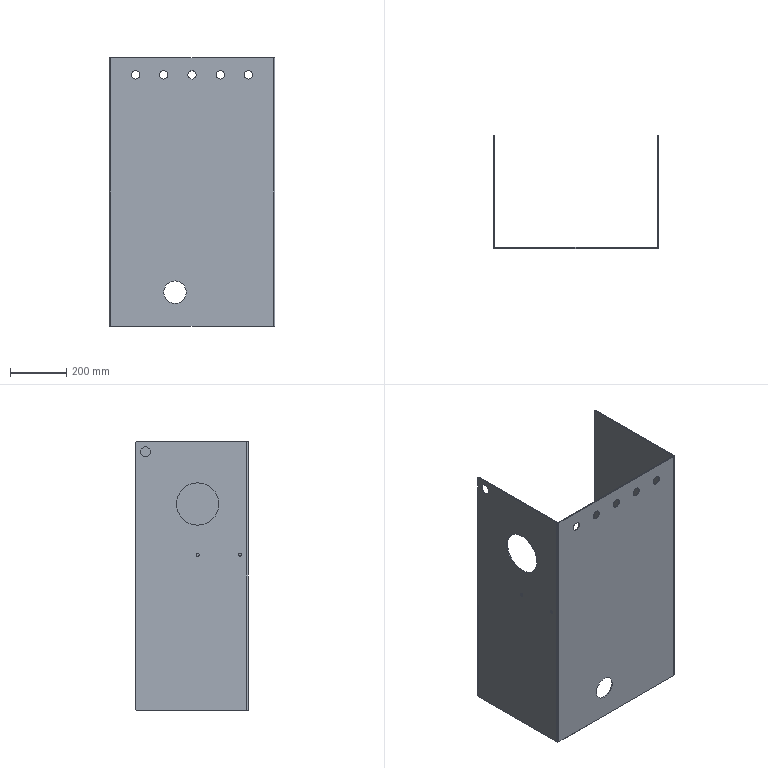Part | SolidWorks | features ICE 4, FlatPattern 1, SMBaseFlange 1, SheetMetal 1 | 1 solid | 48 faces | box 586 x 400 x 950 mm | volume 3763524 mm3 | cylinder 30 | plane 18 | commonest cylinder face diameters 30 x10 6 x6 10.5 x4 12 x2 35 x2 80 x2
STEP:
#1=CARTESIAN_POINT('',(583.,290.,140.));
#2=VERTEX_POINT('',#1);
#3=CARTESIAN_POINT('',(583.,290.,320.));
#4=VERTEX_POINT('',#3);
#5=CARTESIAN_POINT('',(583.,290.,230.));
#6=DIRECTION('',(-1.,0.,0.));
#7=DIRECTION('',(0.,0.,1.));
#8=AXIS2_PLACEMENT_3D('',#5,#6,#7);
#9=CIRCLE('',#8,90.);
#10=EDGE_CURVE('',#2,#4,#9,.T.);
#11=ORIENTED_EDGE('',*,*,#10,.T.);
#12=CARTESIAN_POINT('',(586.,290.,320.));
#13=VERTEX_POINT('',#12);
#14=CARTESIAN_POINT('',(576.,290.,320.));
#15=DIRECTION('',(1.,0.,0.));
#16=VECTOR('',#15,1000.);
#17=LINE('',#14,#16);
#18=EDGE_CURVE('',#4,#13,#17,.T.);
#19=ORIENTED_EDGE('',*,*,#18,.T.);
#20=CARTESIAN_POINT('',(586.,290.,140.));
#21=VERTEX_POINT('',#20);
#22=CARTESIAN_POINT('',(586.,290.,230.));
#23=DIRECTION('',(1.,0.,0.));
#24=DIRECTION('',(0.,0.,-1.));
#25=AXIS2_PLACEMENT_3D('',#22,#23,#24);
#26=CIRCLE('',#25,90.);
#27=EDGE_CURVE('',#13,#21,#26,.T.);
#28=ORIENTED_EDGE('',*,*,#27,.T.);
#29=CARTESIAN_POINT('',(576.,290.,140.));
#30=DIRECTION('',(1.,0.,0.));
#31=VECTOR('',#30,1000.);
#32=LINE('',#29,#31);
#33=EDGE_CURVE('',#2,#21,#32,.T.);
#34=ORIENTED_EDGE('',*,*,#33,.F.);
#35=EDGE_LOOP('',(#11,#19,#28,#34));
#36=FACE_OUTER_BOUND('',#35,.T.);
#37=CARTESIAN_POINT('',(576.,290.,230.));
#38=DIRECTION('',(1.,0.,0.));
#39=DIRECTION('',(0.,0.,-1.));
#40=AXIS2_PLACEMENT_3D('',#37,#38,#39);
#41=CYLINDRICAL_SURFACE('',#40,90.);
#42=ADVANCED_FACE('',(#36),#41,.F.);
#43=CARTESIAN_POINT('',(233.,3.,80.));
#44=VERTEX_POINT('',#43);
#45=CARTESIAN_POINT('',(233.,3.,160.));
#46=VERTEX_POINT('',#45);
#47=CARTESIAN_POINT('',(233.,3.,120.));
#48=DIRECTION('',(0.,1.,0.));
#49=DIRECTION('',(0.,0.,1.));
#50=AXIS2_PLACEMENT_3D('',#47,#48,#49);
#51=CIRCLE('',#50,40.);
#52=EDGE_CURVE('',#44,#46,#51,.T.);
#53=ORIENTED_EDGE('',*,*,#52,.T.);
#54=CARTESIAN_POINT('',(233.,0.,160.));
#55=VERTEX_POINT('',#54);
#56=CARTESIAN_POINT('',(233.,10.,160.));
#57=DIRECTION('',(0.,-1.,0.));
#58=VECTOR('',#57,1000.);
#59=LINE('',#56,#58);
#60=EDGE_CURVE('',#46,#55,#59,.T.);
#61=ORIENTED_EDGE('',*,*,#60,.T.);
#62=CARTESIAN_POINT('',(233.,0.,80.));
#63=VERTEX_POINT('',#62);
#64=CARTESIAN_POINT('',(233.,0.,120.));
#65=DIRECTION('',(0.,-1.,0.));
#66=DIRECTION('',(0.,0.,-1.));
#67=AXIS2_PLACEMENT_3D('',#64,#65,#66);
#68=CIRCLE('',#67,40.);
#69=EDGE_CURVE('',#55,#63,#68,.T.);
#70=ORIENTED_EDGE('',*,*,#69,.T.);
#71=CARTESIAN_POINT('',(233.,10.,80.));
#72=DIRECTION('',(0.,-1.,0.));
#73=VECTOR('',#72,1000.);
#74=LINE('',#71,#73);
#75=EDGE_CURVE('',#44,#63,#74,.T.);
#76=ORIENTED_EDGE('',*,*,#75,.F.);
#77=EDGE_LOOP('',(#53,#61,#70,#76));
#78=FACE_OUTER_BOUND('',#77,.T.);
#79=CARTESIAN_POINT('',(233.,10.,120.));
#80=DIRECTION('',(0.,-1.,0.));
#81=DIRECTION('',(0.,0.,-1.));
#82=AXIS2_PLACEMENT_3D('',#79,#80,#81);
#83=CYLINDRICAL_SURFACE('',#82,40.);
#84=ADVANCED_FACE('',(#78),#83,.F.);
#85=CARTESIAN_POINT('',(493.,3.,875.));
#86=VERTEX_POINT('',#85);
#87=CARTESIAN_POINT('',(493.,3.,905.));
#88=VERTEX_POINT('',#87);
#89=CARTESIAN_POINT('',(493.,3.,890.));
#90=DIRECTION('',(0.,1.,0.));
#91=DIRECTION('',(0.,0.,1.));
#92=AXIS2_PLACEMENT_3D('',#89,#90,#91);
#93=CIRCLE('',#92,15.);
#94=EDGE_CURVE('',#86,#88,#93,.T.);
#95=ORIENTED_EDGE('',*,*,#94,.T.);
#96=CARTESIAN_POINT('',(493.,0.,905.));
#97=VERTEX_POINT('',#96);
#98=CARTESIAN_POINT('',(493.,10.,905.));
#99=DIRECTION('',(0.,-1.,0.));
#100=VECTOR('',#99,1000.);
#101=LINE('',#98,#100);
#102=EDGE_CURVE('',#88,#97,#101,.T.);
#103=ORIENTED_EDGE('',*,*,#102,.T.);
#104=CARTESIAN_POINT('',(493.,0.,875.));
#105=VERTEX_POINT('',#104);
#106=CARTESIAN_POINT('',(493.,0.,890.));
#107=DIRECTION('',(0.,-1.,0.));
#108=DIRECTION('',(0.,0.,-1.));
#109=AXIS2_PLACEMENT_3D('',#106,#107,#108);
#110=CIRCLE('',#109,15.);
#111=EDGE_CURVE('',#97,#105,#110,.T.);
#112=ORIENTED_EDGE('',*,*,#111,.T.);
#113=CARTESIAN_POINT('',(493.,10.,875.));
#114=DIRECTION('',(0.,-1.,0.));
#115=VECTOR('',#114,1000.);
#116=LINE('',#113,#115);
#117=EDGE_CURVE('',#86,#105,#116,.T.);
#118=ORIENTED_EDGE('',*,*,#117,.F.);
#119=EDGE_LOOP('',(#95,#103,#112,#118));
#120=FACE_OUTER_BOUND('',#119,.T.);
#121=CARTESIAN_POINT('',(493.,10.,890.));
#122=DIRECTION('',(0.,-1.,0.));
#123=DIRECTION('',(0.,0.,-1.));
#124=AXIS2_PLACEMENT_3D('',#121,#122,#123);
#125=CYLINDRICAL_SURFACE('',#124,15.);
#126=ADVANCED_FACE('',(#120),#125,.F.);
#127=CARTESIAN_POINT('',(393.,3.,875.));
#128=VERTEX_POINT('',#127);
#129=CARTESIAN_POINT('',(393.,3.,905.));
#130=VERTEX_POINT('',#129);
#131=CARTESIAN_POINT('',(393.,3.,890.));
#132=DIRECTION('',(0.,1.,0.));
#133=DIRECTION('',(0.,0.,1.));
#134=AXIS2_PLACEMENT_3D('',#131,#132,#133);
#135=CIRCLE('',#134,15.);
#136=EDGE_CURVE('',#128,#130,#135,.T.);
#137=ORIENTED_EDGE('',*,*,#136,.T.);
#138=CARTESIAN_POINT('',(393.,0.,905.));
#139=VERTEX_POINT('',#138);
#140=CARTESIAN_POINT('',(393.,10.,905.));
#141=DIRECTION('',(0.,-1.,0.));
#142=VECTOR('',#141,1000.);
#143=LINE('',#140,#142);
#144=EDGE_CURVE('',#130,#139,#143,.T.);
#145=ORIENTED_EDGE('',*,*,#144,.T.);
#146=CARTESIAN_POINT('',(393.,0.,875.));
#147=VERTEX_POINT('',#146);
#148=CARTESIAN_POINT('',(393.,0.,890.));
#149=DIRECTION('',(0.,-1.,0.));
#150=DIRECTION('',(0.,0.,-1.));
#151=AXIS2_PLACEMENT_3D('',#148,#149,#150);
#152=CIRCLE('',#151,15.);
#153=EDGE_CURVE('',#139,#147,#152,.T.);
#154=ORIENTED_EDGE('',*,*,#153,.T.);
#155=CARTESIAN_POINT('',(393.,10.,875.));
#156=DIRECTION('',(0.,-1.,0.));
#157=VECTOR('',#156,1000.);
#158=LINE('',#155,#157);
#159=EDGE_CURVE('',#128,#147,#158,.T.);
#160=ORIENTED_EDGE('',*,*,#159,.F.);
#161=EDGE_LOOP('',(#137,#145,#154,#160));
#162=FACE_OUTER_BOUND('',#161,.T.);
#163=CARTESIAN_POINT('',(393.,10.,890.));
#164=DIRECTION('',(0.,-1.,0.));
#165=DIRECTION('',(0.,0.,-1.));
#166=AXIS2_PLACEMENT_3D('',#163,#164,#165);
#167=CYLINDRICAL_SURFACE('',#166,15.);
#168=ADVANCED_FACE('',(#162),#167,.F.);
#169=CARTESIAN_POINT('',(293.,3.,875.));
#170=VERTEX_POINT('',#169);
#171=CARTESIAN_POINT('',(293.,3.,905.));
#172=VERTEX_POINT('',#171);
#173=CARTESIAN_POINT('',(293.,3.,890.));
#174=DIRECTION('',(0.,1.,0.));
#175=DIRECTION('',(0.,0.,1.));
#176=AXIS2_PLACEMENT_3D('',#173,#174,#175);
#177=CIRCLE('',#176,15.);
#178=EDGE_CURVE('',#170,#172,#177,.T.);
#179=ORIENTED_EDGE('',*,*,#178,.T.);
#180=CARTESIAN_POINT('',(293.,0.,905.));
#181=VERTEX_POINT('',#180);
#182=CARTESIAN_POINT('',(293.,10.,905.));
#183=DIRECTION('',(0.,-1.,0.));
#184=VECTOR('',#183,1000.);
#185=LINE('',#182,#184);
#186=EDGE_CURVE('',#172,#181,#185,.T.);
#187=ORIENTED_EDGE('',*,*,#186,.T.);
#188=CARTESIAN_POINT('',(293.,0.,875.));
#189=VERTEX_POINT('',#188);
#190=CARTESIAN_POINT('',(293.,0.,890.));
#191=DIRECTION('',(0.,-1.,0.));
#192=DIRECTION('',(0.,0.,-1.));
#193=AXIS2_PLACEMENT_3D('',#190,#191,#192);
#194=CIRCLE('',#193,15.);
#195=EDGE_CURVE('',#181,#189,#194,.T.);
#196=ORIENTED_EDGE('',*,*,#195,.T.);
#197=CARTESIAN_POINT('',(293.,10.,875.));
#198=DIRECTION('',(0.,-1.,0.));
#199=VECTOR('',#198,1000.);
#200=LINE('',#197,#199);
#201=EDGE_CURVE('',#170,#189,#200,.T.);
#202=ORIENTED_EDGE('',*,*,#201,.F.);
#203=EDGE_LOOP('',(#179,#187,#196,#202));
#204=FACE_OUTER_BOUND('',#203,.T.);
#205=CARTESIAN_POINT('',(293.,10.,890.));
#206=DIRECTION('',(0.,-1.,0.));
#207=DIRECTION('',(0.,0.,-1.));
#208=AXIS2_PLACEMENT_3D('',#205,#206,#207);
#209=CYLINDRICAL_SURFACE('',#208,15.);
#210=ADVANCED_FACE('',(#204),#209,.F.);
#211=CARTESIAN_POINT('',(193.,3.,875.));
#212=VERTEX_POINT('',#211);
#213=CARTESIAN_POINT('',(193.,3.,905.));
#214=VERTEX_POINT('',#213);
#215=CARTESIAN_POINT('',(193.,3.,890.));
#216=DIRECTION('',(0.,1.,0.));
#217=DIRECTION('',(0.,0.,1.));
#218=AXIS2_PLACEMENT_3D('',#215,#216,#217);
#219=CIRCLE('',#218,15.);
#220=EDGE_CURVE('',#212,#214,#219,.T.);
#221=ORIENTED_EDGE('',*,*,#220,.T.);
#222=CARTESIAN_POINT('',(193.,0.,905.));
#223=VERTEX_POINT('',#222);
#224=CARTESIAN_POINT('',(193.,10.,905.));
#225=DIRECTION('',(0.,-1.,0.));
#226=VECTOR('',#225,1000.);
#227=LINE('',#224,#226);
#228=EDGE_CURVE('',#214,#223,#227,.T.);
#229=ORIENTED_EDGE('',*,*,#228,.T.);
#230=CARTESIAN_POINT('',(193.,0.,875.));
#231=VERTEX_POINT('',#230);
#232=CARTESIAN_POINT('',(193.,0.,890.));
#233=DIRECTION('',(0.,-1.,0.));
#234=DIRECTION('',(0.,0.,-1.));
#235=AXIS2_PLACEMENT_3D('',#232,#233,#234);
#236=CIRCLE('',#235,15.);
#237=EDGE_CURVE('',#223,#231,#236,.T.);
#238=ORIENTED_EDGE('',*,*,#237,.T.);
#239=CARTESIAN_POINT('',(193.,10.,875.));
#240=DIRECTION('',(0.,-1.,0.));
#241=VECTOR('',#240,1000.);
#242=LINE('',#239,#241);
#243=EDGE_CURVE('',#212,#231,#242,.T.);
#244=ORIENTED_EDGE('',*,*,#243,.F.);
#245=EDGE_LOOP('',(#221,#229,#238,#244));
#246=FACE_OUTER_BOUND('',#245,.T.);
#247=CARTESIAN_POINT('',(193.,10.,890.));
#248=DIRECTION('',(0.,-1.,0.));
#249=DIRECTION('',(0.,0.,-1.));
#250=AXIS2_PLACEMENT_3D('',#247,#248,#249);
#251=CYLINDRICAL_SURFACE('',#250,15.);
#252=ADVANCED_FACE('',(#246),#251,.F.);
#253=CARTESIAN_POINT('',(93.,3.,875.));
#254=VERTEX_POINT('',#253);
#255=CARTESIAN_POINT('',(93.,3.,905.));
#256=VERTEX_POINT('',#255);
#257=CARTESIAN_POINT('',(93.,3.,890.));
#258=DIRECTION('',(0.,1.,0.));
#259=DIRECTION('',(0.,0.,1.));
#260=AXIS2_PLACEMENT_3D('',#257,#258,#259);
#261=CIRCLE('',#260,15.);
#262=EDGE_CURVE('',#254,#256,#261,.T.);
#263=ORIENTED_EDGE('',*,*,#262,.T.);
#264=CARTESIAN_POINT('',(93.,0.,905.));
#265=VERTEX_POINT('',#264);
#266=CARTESIAN_POINT('',(93.,10.,905.));
#267=DIRECTION('',(0.,-1.,0.));
#268=VECTOR('',#267,1000.);
#269=LINE('',#266,#268);
#270=EDGE_CURVE('',#256,#265,#269,.T.);
#271=ORIENTED_EDGE('',*,*,#270,.T.);
#272=CARTESIAN_POINT('',(93.,0.,875.));
#273=VERTEX_POINT('',#272);
#274=CARTESIAN_POINT('',(93.,0.,890.));
#275=DIRECTION('',(0.,-1.,0.));
#276=DIRECTION('',(0.,0.,-1.));
#277=AXIS2_PLACEMENT_3D('',#274,#275,#276);
#278=CIRCLE('',#277,15.);
#279=EDGE_CURVE('',#265,#273,#278,.T.);
#280=ORIENTED_EDGE('',*,*,#279,.T.);
#281=CARTESIAN_POINT('',(93.,10.,875.));
#282=DIRECTION('',(0.,-1.,0.));
#283=VECTOR('',#282,1000.);
#284=LINE('',#281,#283);
#285=EDGE_CURVE('',#254,#273,#284,.T.);
#286=ORIENTED_EDGE('',*,*,#285,.F.);
#287=EDGE_LOOP('',(#263,#271,#280,#286));
#288=FACE_OUTER_BOUND('',#287,.T.);
#289=CARTESIAN_POINT('',(93.,10.,890.));
#290=DIRECTION('',(0.,-1.,0.));
#291=DIRECTION('',(0.,0.,-1.));
#292=AXIS2_PLACEMENT_3D('',#289,#290,#291);
#293=CYLINDRICAL_SURFACE('',#292,15.);
#294=ADVANCED_FACE('',(#288),#293,.F.);
#295=CARTESIAN_POINT('',(3.,180.,555.25));
#296=VERTEX_POINT('',#295);
#297=CARTESIAN_POINT('',(3.,180.,544.75));
#298=VERTEX_POINT('',#297);
#299=CARTESIAN_POINT('',(3.,180.,550.));
#300=DIRECTION('',(1.,0.,0.));
#301=DIRECTION('',(0.,0.,-1.));
#302=AXIS2_PLACEMENT_3D('',#299,#300,#301);
#303=CIRCLE('',#302,5.25);
#304=EDGE_CURVE('',#296,#298,#303,.T.);
#305=ORIENTED_EDGE('',*,*,#304,.T.);
#306=CARTESIAN_POINT('',(0.,180.,544.75));
#307=VERTEX_POINT('',#306);
#308=CARTESIAN_POINT('',(10.,180.,544.75));
#309=DIRECTION('',(-1.,0.,0.));
#310=VECTOR('',#309,1000.);
#311=LINE('',#308,#310);
#312=EDGE_CURVE('',#298,#307,#311,.T.);
#313=ORIENTED_EDGE('',*,*,#312,.T.);
#314=CARTESIAN_POINT('',(0.,180.,555.25));
#315=VERTEX_POINT('',#314);
#316=CARTESIAN_POINT('',(0.,180.,550.));
#317=DIRECTION('',(-1.,0.,0.));
#318=DIRECTION('',(0.,0.,1.));
#319=AXIS2_PLACEMENT_3D('',#316,#317,#318);
#320=CIRCLE('',#319,5.25);
#321=EDGE_CURVE('',#307,#315,#320,.T.);
#322=ORIENTED_EDGE('',*,*,#321,.T.);
#323=CARTESIAN_POINT('',(10.,180.,555.25));
#324=DIRECTION('',(-1.,0.,0.));
#325=VECTOR('',#324,1000.);
#326=LINE('',#323,#325);
#327=EDGE_CURVE('',#296,#315,#326,.T.);
#328=ORIENTED_EDGE('',*,*,#327,.F.);
#329=EDGE_LOOP('',(#305,#313,#322,#328));
#330=FACE_OUTER_BOUND('',#329,.T.);
#331=CARTESIAN_POINT('',(10.,180.,550.));
#332=DIRECTION('',(-1.,0.,0.));
#333=DIRECTION('',(0.,0.,1.));
#334=AXIS2_PLACEMENT_3D('',#331,#332,#333);
#335=CYLINDRICAL_SURFACE('',#334,5.25);
#336=ADVANCED_FACE('',(#330),#335,.F.);
#337=CARTESIAN_POINT('',(3.,30.,555.25));
#338=VERTEX_POINT('',#337);
#339=CARTESIAN_POINT('',(3.,30.,544.75));
#340=VERTEX_POINT('',#339);
#341=CARTESIAN_POINT('',(3.,30.,550.));
#342=DIRECTION('',(1.,0.,0.));
#343=DIRECTION('',(0.,0.,-1.));
#344=AXIS2_PLACEMENT_3D('',#341,#342,#343);
#345=CIRCLE('',#344,5.25);
#346=EDGE_CURVE('',#338,#340,#345,.T.);
#347=ORIENTED_EDGE('',*,*,#346,.T.);
#348=CARTESIAN_POINT('',(0.,30.,544.75));
#349=VERTEX_POINT('',#348);
#350=CARTESIAN_POINT('',(10.,30.,544.75));
#351=DIRECTION('',(-1.,0.,0.));
#352=VECTOR('',#351,1000.);
#353=LINE('',#350,#352);
#354=EDGE_CURVE('',#340,#349,#353,.T.);
#355=ORIENTED_EDGE('',*,*,#354,.T.);
#356=CARTESIAN_POINT('',(0.,30.,555.25));
#357=VERTEX_POINT('',#356);
#358=CARTESIAN_POINT('',(0.,30.,550.));
#359=DIRECTION('',(-1.,0.,0.));
#360=DIRECTION('',(0.,0.,1.));
#361=AXIS2_PLACEMENT_3D('',#358,#359,#360);
#362=CIRCLE('',#361,5.25);
#363=EDGE_CURVE('',#349,#357,#362,.T.);
#364=ORIENTED_EDGE('',*,*,#363,.T.);
#365=CARTESIAN_POINT('',(10.,30.,555.25));
#366=DIRECTION('',(-1.,0.,0.));
#367=VECTOR('',#366,1000.);
#368=LINE('',#365,#367);
#369=EDGE_CURVE('',#338,#357,#368,.T.);
#370=ORIENTED_EDGE('',*,*,#369,.F.);
#371=EDGE_LOOP('',(#347,#355,#364,#370));
#372=FACE_OUTER_BOUND('',#371,.T.);
#373=CARTESIAN_POINT('',(10.,30.,550.));
#374=DIRECTION('',(-1.,0.,0.));
#375=DIRECTION('',(0.,0.,1.));
#376=AXIS2_PLACEMENT_3D('',#373,#374,#375);
#377=CYLINDRICAL_SURFACE('',#376,5.25);
#378=ADVANCED_FACE('',(#372),#377,.F.);
#379=CARTESIAN_POINT('',(3.,365.,932.5));
#380=VERTEX_POINT('',#379);
#381=CARTESIAN_POINT('',(3.,365.,897.5));
#382=VERTEX_POINT('',#381);
#383=CARTESIAN_POINT('',(3.,365.,915.));
#384=DIRECTION('',(1.,0.,0.));
#385=DIRECTION('',(0.,0.,-1.));
#386=AXIS2_PLACEMENT_3D('',#383,#384,#385);
#387=CIRCLE('',#386,17.5);
#388=EDGE_CURVE('',#380,#382,#387,.T.);
#389=ORIENTED_EDGE('',*,*,#388,.T.);
#390=CARTESIAN_POINT('',(0.,365.,897.5));
#391=VERTEX_POINT('',#390);
#392=CARTESIAN_POINT('',(10.,365.,897.5));
#393=DIRECTION('',(-1.,0.,0.));
#394=VECTOR('',#393,1000.);
#395=LINE('',#392,#394);
#396=EDGE_CURVE('',#382,#391,#395,.T.);
#397=ORIENTED_EDGE('',*,*,#396,.T.);
#398=CARTESIAN_POINT('',(0.,365.,932.5));
#399=VERTEX_POINT('',#398);
#400=CARTESIAN_POINT('',(0.,365.,915.));
#401=DIRECTION('',(-1.,0.,0.));
#402=DIRECTION('',(0.,0.,1.));
#403=AXIS2_PLACEMENT_3D('',#400,#401,#402);
#404=CIRCLE('',#403,17.5);
#405=EDGE_CURVE('',#391,#399,#404,.T.);
#406=ORIENTED_EDGE('',*,*,#405,.T.);
#407=CARTESIAN_POINT('',(10.,365.,932.5));
#408=DIRECTION('',(-1.,0.,0.));
#409=VECTOR('',#408,1000.);
#410=LINE('',#407,#409);
#411=EDGE_CURVE('',#380,#399,#410,.T.);
#412=ORIENTED_EDGE('',*,*,#411,.F.);
#413=EDGE_LOOP('',(#389,#397,#406,#412));
#414=FACE_OUTER_BOUND('',#413,.T.);
#415=CARTESIAN_POINT('',(10.,365.,915.));
#416=DIRECTION('',(-1.,0.,0.));
#417=DIRECTION('',(0.,0.,1.));
#418=AXIS2_PLACEMENT_3D('',#415,#416,#417);
#419=CYLINDRICAL_SURFACE('',#418,17.5);
#420=ADVANCED_FACE('',(#414),#419,.F.);
#421=CARTESIAN_POINT('',(3.,180.,805.));
#422=VERTEX_POINT('',#421);
#423=CARTESIAN_POINT('',(3.,180.,655.));
#424=VERTEX_POINT('',#423);
#425=CARTESIAN_POINT('',(3.,180.,730.));
#426=DIRECTION('',(1.,0.,0.));
#427=DIRECTION('',(0.,0.,-1.));
#428=AXIS2_PLACEMENT_3D('',#425,#426,#427);
#429=CIRCLE('',#428,75.);
#430=EDGE_CURVE('',#422,#424,#429,.T.);
#431=ORIENTED_EDGE('',*,*,#430,.T.);
#432=CARTESIAN_POINT('',(0.,180.,655.));
#433=VERTEX_POINT('',#432);
#434=CARTESIAN_POINT('',(10.,180.,655.));
#435=DIRECTION('',(-1.,0.,0.));
#436=VECTOR('',#435,1000.);
#437=LINE('',#434,#436);
#438=EDGE_CURVE('',#424,#433,#437,.T.);
#439=ORIENTED_EDGE('',*,*,#438,.T.);
#440=CARTESIAN_POINT('',(0.,180.,805.));
#441=VERTEX_POINT('',#440);
#442=CARTESIAN_POINT('',(0.,180.,730.));
#443=DIRECTION('',(-1.,0.,0.));
#444=DIRECTION('',(0.,0.,1.));
#445=AXIS2_PLACEMENT_3D('',#442,#443,#444);
#446=CIRCLE('',#445,75.);
#447=EDGE_CURVE('',#433,#441,#446,.T.);
#448=ORIENTED_EDGE('',*,*,#447,.T.);
#449=CARTESIAN_POINT('',(10.,180.,805.));
#450=DIRECTION('',(-1.,0.,0.));
#451=VECTOR('',#450,1000.);
#452=LINE('',#449,#451);
#453=EDGE_CURVE('',#422,#441,#452,.T.);
#454=ORIENTED_EDGE('',*,*,#453,.F.);
#455=EDGE_LOOP('',(#431,#439,#448,#454));
#456=FACE_OUTER_BOUND('',#455,.T.);
#457=CARTESIAN_POINT('',(10.,180.,730.));
#458=DIRECTION('',(-1.,0.,0.));
#459=DIRECTION('',(0.,0.,1.));
#460=AXIS2_PLACEMENT_3D('',#457,#458,#459);
#461=CYLINDRICAL_SURFACE('',#460,75.);
#462=ADVANCED_FACE('',(#456),#461,.F.);
#463=CARTESIAN_POINT('',(586.,290.,230.));
#464=DIRECTION('',(1.,0.,0.));
#465=DIRECTION('',(0.,0.,-1.));
#466=AXIS2_PLACEMENT_3D('',#463,#464,#465);
#467=CIRCLE('',#466,90.);
#468=EDGE_CURVE('',#21,#13,#467,.T.);
#469=ORIENTED_EDGE('',*,*,#468,.F.);
#470=ORIENTED_EDGE('',*,*,#27,.F.);
#471=EDGE_LOOP('',(#469,#470));
#472=FACE_BOUND('',#471,.T.);
#473=CARTESIAN_POINT('',(586.,397.,0.));
#474=VERTEX_POINT('',#473);
#475=CARTESIAN_POINT('',(586.,400.,3.));
#476=VERTEX_POINT('',#475);
#477=CARTESIAN_POINT('',(586.,397.,3.));
#478=DIRECTION('',(1.,0.,0.));
#479=DIRECTION('',(0.,0.,1.));
#480=AXIS2_PLACEMENT_3D('',#477,#478,#479);
#481=CIRCLE('',#480,3.);
#482=EDGE_CURVE('',#474,#476,#481,.T.);
#483=ORIENTED_EDGE('',*,*,#482,.T.);
#484=CARTESIAN_POINT('',(586.,400.,947.));
#485=VERTEX_POINT('',#484);
#486=CARTESIAN_POINT('',(586.,400.,950.));
#487=DIRECTION('',(0.,0.,-1.));
#488=VECTOR('',#487,1000.);
#489=LINE('',#486,#488);
#490=EDGE_CURVE('',#485,#476,#489,.T.);
#491=ORIENTED_EDGE('',*,*,#490,.F.);
#492=CARTESIAN_POINT('',(586.,397.,950.));
#493=VERTEX_POINT('',#492);
#494=CARTESIAN_POINT('',(586.,397.,947.));
#495=DIRECTION('',(1.,0.,0.));
#496=DIRECTION('',(0.,0.,1.));
#497=AXIS2_PLACEMENT_3D('',#494,#495,#496);
#498=CIRCLE('',#497,3.);
#499=EDGE_CURVE('',#485,#493,#498,.T.);
#500=ORIENTED_EDGE('',*,*,#499,.T.);
#501=CARTESIAN_POINT('',(586.,6.,950.));
#502=VERTEX_POINT('',#501);
#503=CARTESIAN_POINT('',(586.,0.,950.));
#504=DIRECTION('',(0.,1.,0.));
#505=VECTOR('',#504,1000.);
#506=LINE('',#503,#505);
#507=EDGE_CURVE('',#502,#493,#506,.T.);
#508=ORIENTED_EDGE('',*,*,#507,.F.);
#509=CARTESIAN_POINT('',(586.,6.,0.));
#510=VERTEX_POINT('',#509);
#511=CARTESIAN_POINT('',(586.,6.,950.));
#512=DIRECTION('',(0.,0.,-1.));
#513=VECTOR('',#512,1000.);
#514=LINE('',#511,#513);
#515=EDGE_CURVE('',#502,#510,#514,.T.);
#516=ORIENTED_EDGE('',*,*,#515,.T.);
#517=CARTESIAN_POINT('',(586.,0.,0.));
#518=DIRECTION('',(0.,1.,0.));
#519=VECTOR('',#518,1000.);
#520=LINE('',#517,#519);
#521=EDGE_CURVE('',#510,#474,#520,.T.);
#522=ORIENTED_EDGE('',*,*,#521,.T.);
#523=EDGE_LOOP('',(#483,#491,#500,#508,#516,#522));
#524=FACE_OUTER_BOUND('',#523,.T.);
#525=CARTESIAN_POINT('',(586.,0.,950.));
#526=DIRECTION('',(-1.,0.,0.));
#527=DIRECTION('',(0.,0.,1.));
#528=AXIS2_PLACEMENT_3D('',#525,#526,#527);
#529=PLANE('',#528);
#530=ADVANCED_FACE('',(#472,#524),#529,.F.);
#531=ORIENTED_EDGE('',*,*,#10,.F.);
#532=CARTESIAN_POINT('',(583.,290.,230.));
#533=DIRECTION('',(-1.,0.,0.));
#534=DIRECTION('',(0.,0.,1.));
#535=AXIS2_PLACEMENT_3D('',#532,#533,#534);
#536=CIRCLE('',#535,90.);
#537=EDGE_CURVE('',#4,#2,#536,.T.);
#538=ORIENTED_EDGE('',*,*,#537,.F.);
#539=EDGE_LOOP('',(#531,#538));
#540=FACE_BOUND('',#539,.T.);
#541=CARTESIAN_POINT('',(583.,400.,947.));
#542=VERTEX_POINT('',#541);
#543=CARTESIAN_POINT('',(583.,400.,3.));
#544=VERTEX_POINT('',#543);
#545=CARTESIAN_POINT('',(583.,400.,950.));
#546=DIRECTION('',(0.,0.,-1.));
#547=VECTOR('',#546,1000.);
#548=LINE('',#545,#547);
#549=EDGE_CURVE('',#542,#544,#548,.T.);
#550=ORIENTED_EDGE('',*,*,#549,.T.);
#551=CARTESIAN_POINT('',(583.,397.,0.));
#552=VERTEX_POINT('',#551);
#553=CARTESIAN_POINT('',(583.,397.,3.));
#554=DIRECTION('',(1.,0.,0.));
#555=DIRECTION('',(0.,0.,1.));
#556=AXIS2_PLACEMENT_3D('',#553,#554,#555);
#557=CIRCLE('',#556,3.);
#558=EDGE_CURVE('',#552,#544,#557,.T.);
#559=ORIENTED_EDGE('',*,*,#558,.F.);
#560=CARTESIAN_POINT('',(583.,6.,0.));
#561=VERTEX_POINT('',#560);
#562=CARTESIAN_POINT('',(583.,0.,0.));
#563=DIRECTION('',(0.,1.,0.));
#564=VECTOR('',#563,1000.);
#565=LINE('',#562,#564);
#566=EDGE_CURVE('',#561,#552,#565,.T.);
#567=ORIENTED_EDGE('',*,*,#566,.F.);
#568=CARTESIAN_POINT('',(583.,6.,950.));
#569=VERTEX_POINT('',#568);
#570=CARTESIAN_POINT('',(583.,6.,950.));
#571=DIRECTION('',(0.,0.,-1.));
#572=VECTOR('',#571,1000.);
#573=LINE('',#570,#572);
#574=EDGE_CURVE('',#569,#561,#573,.T.);
#575=ORIENTED_EDGE('',*,*,#574,.F.);
#576=CARTESIAN_POINT('',(583.,397.,950.));
#577=VERTEX_POINT('',#576);
#578=CARTESIAN_POINT('',(583.,0.,950.));
#579=DIRECTION('',(0.,1.,0.));
#580=VECTOR('',#579,1000.);
#581=LINE('',#578,#580);
#582=EDGE_CURVE('',#569,#577,#581,.T.);
#583=ORIENTED_EDGE('',*,*,#582,.T.);
#584=CARTESIAN_POINT('',(583.,397.,947.));
#585=DIRECTION('',(1.,0.,0.));
#586=DIRECTION('',(0.,0.,1.));
#587=AXIS2_PLACEMENT_3D('',#584,#585,#586);
#588=CIRCLE('',#587,3.);
#589=EDGE_CURVE('',#542,#577,#588,.T.);
#590=ORIENTED_EDGE('',*,*,#589,.F.);
#591=EDGE_LOOP('',(#550,#559,#567,#575,#583,#590));
#592=FACE_OUTER_BOUND('',#591,.T.);
#593=CARTESIAN_POINT('',(583.,0.,950.));
#594=DIRECTION('',(-1.,0.,0.));
#595=DIRECTION('',(0.,0.,1.));
#596=AXIS2_PLACEMENT_3D('',#593,#594,#595);
#597=PLANE('',#596);
#598=ADVANCED_FACE('',(#540,#592),#597,.T.);
#599=ORIENTED_EDGE('',*,*,#490,.T.);
#600=CARTESIAN_POINT('',(583.,400.,3.));
#601=DIRECTION('',(1.,0.,0.));
#602=VECTOR('',#601,1000.);
#603=LINE('',#600,#602);
#604=EDGE_CURVE('',#544,#476,#603,.T.);
#605=ORIENTED_EDGE('',*,*,#604,.F.);
#606=ORIENTED_EDGE('',*,*,#549,.F.);
#607=CARTESIAN_POINT('',(583.,400.,947.));
#608=DIRECTION('',(1.,0.,0.));
#609=VECTOR('',#608,1000.);
#610=LINE('',#607,#609);
#611=EDGE_CURVE('',#542,#485,#610,.T.);
#612=ORIENTED_EDGE('',*,*,#611,.T.);
#613=EDGE_LOOP('',(#599,#605,#606,#612));
#614=FACE_OUTER_BOUND('',#613,.T.);
#615=CARTESIAN_POINT('',(583.,400.,950.));
#616=DIRECTION('',(0.,1.,0.));
#617=DIRECTION('',(0.,0.,1.));
#618=AXIS2_PLACEMENT_3D('',#615,#616,#617);
#619=PLANE('',#618);
#620=ADVANCED_FACE('',(#614),#619,.T.);
#621=ORIENTED_EDGE('',*,*,#304,.F.);
#622=CARTESIAN_POINT('',(3.,180.,550.));
#623=DIRECTION('',(1.,0.,0.));
#624=DIRECTION('',(0.,0.,-1.));
#625=AXIS2_PLACEMENT_3D('',#622,#623,#624);
#626=CIRCLE('',#625,5.25);
#627=EDGE_CURVE('',#298,#296,#626,.T.);
#628=ORIENTED_EDGE('',*,*,#627,.F.);
#629=EDGE_LOOP('',(#621,#628));
#630=FACE_BOUND('',#629,.T.);
#631=ORIENTED_EDGE('',*,*,#346,.F.);
#632=CARTESIAN_POINT('',(3.,30.,550.));
#633=DIRECTION('',(1.,0.,0.));
#634=DIRECTION('',(0.,0.,-1.));
#635=AXIS2_PLACEMENT_3D('',#632,#633,#634);
#636=CIRCLE('',#635,5.25);
#637=EDGE_CURVE('',#340,#338,#636,.T.);
#638=ORIENTED_EDGE('',*,*,#637,.F.);
#639=EDGE_LOOP('',(#631,#638));
#640=FACE_BOUND('',#639,.T.);
#641=ORIENTED_EDGE('',*,*,#388,.F.);
#642=CARTESIAN_POINT('',(3.,365.,915.));
#643=DIRECTION('',(1.,0.,0.));
#644=DIRECTION('',(0.,0.,-1.));
#645=AXIS2_PLACEMENT_3D('',#642,#643,#644);
#646=CIRCLE('',#645,17.5);
#647=EDGE_CURVE('',#382,#380,#646,.T.);
#648=ORIENTED_EDGE('',*,*,#647,.F.);
#649=EDGE_LOOP('',(#641,#648));
#650=FACE_BOUND('',#649,.T.);
#651=ORIENTED_EDGE('',*,*,#430,.F.);
#652=CARTESIAN_POINT('',(3.,180.,730.));
#653=DIRECTION('',(1.,0.,0.));
#654=DIRECTION('',(0.,0.,-1.));
#655=AXIS2_PLACEMENT_3D('',#652,#653,#654);
#656=CIRCLE('',#655,75.);
#657=EDGE_CURVE('',#424,#422,#656,.T.);
#658=ORIENTED_EDGE('',*,*,#657,.F.);
#659=EDGE_LOOP('',(#651,#658));
#660=FACE_BOUND('',#659,.T.);
#661=CARTESIAN_POINT('',(3.,397.,0.));
#662=VERTEX_POINT('',#661);
#663=CARTESIAN_POINT('',(3.,6.,0.));
#664=VERTEX_POINT('',#663);
#665=CARTESIAN_POINT('',(3.,0.,0.));
#666=DIRECTION('',(0.,-1.,0.));
#667=VECTOR('',#666,1000.);
#668=LINE('',#665,#667);
#669=EDGE_CURVE('',#662,#664,#668,.T.);
#670=ORIENTED_EDGE('',*,*,#669,.F.);
#671=CARTESIAN_POINT('',(3.,400.,3.));
#672=VERTEX_POINT('',#671);
#673=CARTESIAN_POINT('',(3.,397.,3.));
#674=DIRECTION('',(-1.,0.,0.));
#675=DIRECTION('',(0.,0.,-1.));
#676=AXIS2_PLACEMENT_3D('',#673,#674,#675);
#677=CIRCLE('',#676,3.);
#678=EDGE_CURVE('',#672,#662,#677,.T.);
#679=ORIENTED_EDGE('',*,*,#678,.F.);
#680=CARTESIAN_POINT('',(3.,400.,947.));
#681=VERTEX_POINT('',#680);
#682=CARTESIAN_POINT('',(3.,400.,950.));
#683=DIRECTION('',(0.,0.,-1.));
#684=VECTOR('',#683,1000.);
#685=LINE('',#682,#684);
#686=EDGE_CURVE('',#681,#672,#685,.T.);
#687=ORIENTED_EDGE('',*,*,#686,.F.);
#688=CARTESIAN_POINT('',(3.,397.,950.));
#689=VERTEX_POINT('',#688);
#690=CARTESIAN_POINT('',(3.,397.,947.));
#691=DIRECTION('',(-1.,0.,0.));
#692=DIRECTION('',(0.,0.,-1.));
#693=AXIS2_PLACEMENT_3D('',#690,#691,#692);
#694=CIRCLE('',#693,3.);
#695=EDGE_CURVE('',#689,#681,#694,.T.);
#696=ORIENTED_EDGE('',*,*,#695,.F.);
#697=CARTESIAN_POINT('',(3.,6.,950.));
#698=VERTEX_POINT('',#697);
#699=CARTESIAN_POINT('',(3.,0.,950.));
#700=DIRECTION('',(0.,-1.,0.));
#701=VECTOR('',#700,1000.);
#702=LINE('',#699,#701);
#703=EDGE_CURVE('',#689,#698,#702,.T.);
#704=ORIENTED_EDGE('',*,*,#703,.T.);
#705=CARTESIAN_POINT('',(3.,6.,950.));
#706=DIRECTION('',(0.,0.,-1.));
#707=VECTOR('',#706,1000.);
#708=LINE('',#705,#707);
#709=EDGE_CURVE('',#698,#664,#708,.T.);
#710=ORIENTED_EDGE('',*,*,#709,.T.);
#711=EDGE_LOOP('',(#670,#679,#687,#696,#704,#710));
#712=FACE_OUTER_BOUND('',#711,.T.);
#713=CARTESIAN_POINT('',(3.,0.,950.));
#714=DIRECTION('',(1.,0.,0.));
#715=DIRECTION('',(0.,0.,-1.));
#716=AXIS2_PLACEMENT_3D('',#713,#714,#715);
#717=PLANE('',#716);
#718=ADVANCED_FACE('',(#630,#640,#650,#660,#712),#717,.T.);
#719=CARTESIAN_POINT('',(0.,180.,550.));
#720=DIRECTION('',(-1.,0.,0.));
#721=DIRECTION('',(0.,0.,1.));
#722=AXIS2_PLACEMENT_3D('',#719,#720,#721);
#723=CIRCLE('',#722,5.25);
#724=EDGE_CURVE('',#315,#307,#723,.T.);
#725=ORIENTED_EDGE('',*,*,#724,.F.);
#726=ORIENTED_EDGE('',*,*,#321,.F.);
#727=EDGE_LOOP('',(#725,#726));
#728=FACE_BOUND('',#727,.T.);
#729=CARTESIAN_POINT('',(0.,30.,550.));
#730=DIRECTION('',(-1.,0.,0.));
#731=DIRECTION('',(0.,0.,1.));
#732=AXIS2_PLACEMENT_3D('',#729,#730,#731);
#733=CIRCLE('',#732,5.25);
#734=EDGE_CURVE('',#357,#349,#733,.T.);
#735=ORIENTED_EDGE('',*,*,#734,.F.);
#736=ORIENTED_EDGE('',*,*,#363,.F.);
#737=EDGE_LOOP('',(#735,#736));
#738=FACE_BOUND('',#737,.T.);
#739=CARTESIAN_POINT('',(0.,365.,915.));
#740=DIRECTION('',(-1.,0.,0.));
#741=DIRECTION('',(0.,0.,1.));
#742=AXIS2_PLACEMENT_3D('',#739,#740,#741);
#743=CIRCLE('',#742,17.5);
#744=EDGE_CURVE('',#399,#391,#743,.T.);
#745=ORIENTED_EDGE('',*,*,#744,.F.);
#746=ORIENTED_EDGE('',*,*,#405,.F.);
#747=EDGE_LOOP('',(#745,#746));
#748=FACE_BOUND('',#747,.T.);
#749=CARTESIAN_POINT('',(0.,180.,730.));
#750=DIRECTION('',(-1.,0.,0.));
#751=DIRECTION('',(0.,0.,1.));
#752=AXIS2_PLACEMENT_3D('',#749,#750,#751);
#753=CIRCLE('',#752,75.);
#754=EDGE_CURVE('',#441,#433,#753,.T.);
#755=ORIENTED_EDGE('',*,*,#754,.F.);
#756=ORIENTED_EDGE('',*,*,#447,.F.);
#757=EDGE_LOOP('',(#755,#756));
#758=FACE_BOUND('',#757,.T.);
#759=CARTESIAN_POINT('',(0.,400.,3.));
#760=VERTEX_POINT('',#759);
#761=CARTESIAN_POINT('',(0.,397.,0.));
#762=VERTEX_POINT('',#761);
#763=CARTESIAN_POINT('',(0.,397.,3.));
#764=DIRECTION('',(-1.,0.,0.));
#765=DIRECTION('',(0.,0.,-1.));
#766=AXIS2_PLACEMENT_3D('',#763,#764,#765);
#767=CIRCLE('',#766,3.);
#768=EDGE_CURVE('',#760,#762,#767,.T.);
#769=ORIENTED_EDGE('',*,*,#768,.T.);
#770=CARTESIAN_POINT('',(0.,6.,0.));
#771=VERTEX_POINT('',#770);
#772=CARTESIAN_POINT('',(0.,0.,0.));
#773=DIRECTION('',(0.,-1.,0.));
#774=VECTOR('',#773,1000.);
#775=LINE('',#772,#774);
#776=EDGE_CURVE('',#762,#771,#775,.T.);
#777=ORIENTED_EDGE('',*,*,#776,.T.);
#778=CARTESIAN_POINT('',(0.,6.,950.));
#779=VERTEX_POINT('',#778);
#780=CARTESIAN_POINT('',(0.,6.,950.));
#781=DIRECTION('',(0.,0.,-1.));
#782=VECTOR('',#781,1000.);
#783=LINE('',#780,#782);
#784=EDGE_CURVE('',#779,#771,#783,.T.);
#785=ORIENTED_EDGE('',*,*,#784,.F.);
#786=CARTESIAN_POINT('',(0.,397.,950.));
#787=VERTEX_POINT('',#786);
#788=CARTESIAN_POINT('',(0.,0.,950.));
#789=DIRECTION('',(0.,-1.,0.));
#790=VECTOR('',#789,1000.);
#791=LINE('',#788,#790);
#792=EDGE_CURVE('',#787,#779,#791,.T.);
#793=ORIENTED_EDGE('',*,*,#792,.F.);
#794=CARTESIAN_POINT('',(0.,400.,947.));
#795=VERTEX_POINT('',#794);
#796=CARTESIAN_POINT('',(0.,397.,947.));
#797=DIRECTION('',(-1.,0.,0.));
#798=DIRECTION('',(0.,0.,-1.));
#799=AXIS2_PLACEMENT_3D('',#796,#797,#798);
#800=CIRCLE('',#799,3.);
#801=EDGE_CURVE('',#787,#795,#800,.T.);
#802=ORIENTED_EDGE('',*,*,#801,.T.);
#803=CARTESIAN_POINT('',(0.,400.,950.));
#804=DIRECTION('',(0.,0.,-1.));
#805=VECTOR('',#804,1000.);
#806=LINE('',#803,#805);
#807=EDGE_CURVE('',#795,#760,#806,.T.);
#808=ORIENTED_EDGE('',*,*,#807,.T.);
#809=EDGE_LOOP('',(#769,#777,#785,#793,#802,#808));
#810=FACE_OUTER_BOUND('',#809,.T.);
#811=CARTESIAN_POINT('',(0.,0.,950.));
#812=DIRECTION('',(1.,0.,0.));
#813=DIRECTION('',(0.,0.,-1.));
#814=AXIS2_PLACEMENT_3D('',#811,#812,#813);
#815=PLANE('',#814);
#816=ADVANCED_FACE('',(#728,#738,#748,#758,#810),#815,.F.);
#817=ORIENTED_EDGE('',*,*,#507,.T.);
#818=CARTESIAN_POINT('',(583.,397.,950.));
#819=DIRECTION('',(1.,0.,0.));
#820=VECTOR('',#819,1000.);
#821=LINE('',#818,#820);
#822=EDGE_CURVE('',#577,#493,#821,.T.);
#823=ORIENTED_EDGE('',*,*,#822,.F.);
#824=ORIENTED_EDGE('',*,*,#582,.F.);
#825=CARTESIAN_POINT('',(583.,6.,950.));
#826=DIRECTION('',(1.,0.,0.));
#827=VECTOR('',#826,1000.);
#828=LINE('',#825,#827);
#829=EDGE_CURVE('',#569,#502,#828,.T.);
#830=ORIENTED_EDGE('',*,*,#829,.T.);
#831=EDGE_LOOP('',(#817,#823,#824,#830));
#832=FACE_OUTER_BOUND('',#831,.T.);
#833=CARTESIAN_POINT('',(580.,6.,950.));
#834=DIRECTION('',(0.,0.,1.));
#835=DIRECTION('',(1.,0.,0.));
#836=AXIS2_PLACEMENT_3D('',#833,#834,#835);
#837=PLANE('',#836);
#838=ADVANCED_FACE('',(#832),#837,.T.);
#839=CARTESIAN_POINT('',(3.,400.,3.));
#840=DIRECTION('',(-1.,0.,0.));
#841=VECTOR('',#840,1000.);
#842=LINE('',#839,#841);
#843=EDGE_CURVE('',#672,#760,#842,.T.);
#844=ORIENTED_EDGE('',*,*,#843,.T.);
#845=ORIENTED_EDGE('',*,*,#807,.F.);
#846=CARTESIAN_POINT('',(3.,400.,947.));
#847=DIRECTION('',(-1.,0.,0.));
#848=VECTOR('',#847,1000.);
#849=LINE('',#846,#848);
#850=EDGE_CURVE('',#681,#795,#849,.T.);
#851=ORIENTED_EDGE('',*,*,#850,.F.);
#852=ORIENTED_EDGE('',*,*,#686,.T.);
#853=EDGE_LOOP('',(#844,#845,#851,#852));
#854=FACE_OUTER_BOUND('',#853,.T.);
#855=CARTESIAN_POINT('',(0.,400.,950.));
#856=DIRECTION('',(0.,1.,0.));
#857=DIRECTION('',(0.,0.,1.));
#858=AXIS2_PLACEMENT_3D('',#855,#856,#857);
#859=PLANE('',#858);
#860=ADVANCED_FACE('',(#854),#859,.T.);
#861=CARTESIAN_POINT('',(0.,6.,950.));
#862=DIRECTION('',(1.,0.,0.));
#863=VECTOR('',#862,1000.);
#864=LINE('',#861,#863);
#865=EDGE_CURVE('',#779,#698,#864,.T.);
#866=ORIENTED_EDGE('',*,*,#865,.F.);
#867=CARTESIAN_POINT('',(6.,0.,950.));
#868=VERTEX_POINT('',#867);
#869=CARTESIAN_POINT('',(6.,6.,950.));
#870=DIRECTION('',(0.,0.,1.));
#871=DIRECTION('',(-1.,0.,0.));
#872=AXIS2_PLACEMENT_3D('',#869,#870,#871);
#873=CIRCLE('',#872,6.);
#874=EDGE_CURVE('',#779,#868,#873,.T.);
#875=ORIENTED_EDGE('',*,*,#874,.T.);
#876=CARTESIAN_POINT('',(6.,3.,950.));
#877=VERTEX_POINT('',#876);
#878=CARTESIAN_POINT('',(6.,3.,950.));
#879=DIRECTION('',(0.,-1.,0.));
#880=VECTOR('',#879,1000.);
#881=LINE('',#878,#880);
#882=EDGE_CURVE('',#877,#868,#881,.T.);
#883=ORIENTED_EDGE('',*,*,#882,.F.);
#884=CARTESIAN_POINT('',(6.,6.,950.));
#885=DIRECTION('',(0.,0.,1.));
#886=DIRECTION('',(1.,0.,0.));
#887=AXIS2_PLACEMENT_3D('',#884,#885,#886);
#888=CIRCLE('',#887,3.);
#889=EDGE_CURVE('',#698,#877,#888,.T.);
#890=ORIENTED_EDGE('',*,*,#889,.F.);
#891=EDGE_LOOP('',(#866,#875,#883,#890));
#892=FACE_OUTER_BOUND('',#891,.T.);
#893=CARTESIAN_POINT('',(0.,6.,950.));
#894=DIRECTION('',(0.,0.,1.));
#895=DIRECTION('',(1.,0.,0.));
#896=AXIS2_PLACEMENT_3D('',#893,#894,#895);
#897=PLANE('',#896);
#898=ADVANCED_FACE('',(#892),#897,.T.);
#899=CARTESIAN_POINT('',(3.,397.,950.));
#900=DIRECTION('',(-1.,0.,0.));
#901=VECTOR('',#900,1000.);
#902=LINE('',#899,#901);
#903=EDGE_CURVE('',#689,#787,#902,.T.);
#904=ORIENTED_EDGE('',*,*,#903,.T.);
#905=ORIENTED_EDGE('',*,*,#792,.T.);
#906=ORIENTED_EDGE('',*,*,#865,.T.);
#907=ORIENTED_EDGE('',*,*,#703,.F.);
#908=EDGE_LOOP('',(#904,#905,#906,#907));
#909=FACE_OUTER_BOUND('',#908,.T.);
#910=CARTESIAN_POINT('',(6.,3.,950.));
#911=DIRECTION('',(0.,0.,1.));
#912=DIRECTION('',(1.,0.,0.));
#913=AXIS2_PLACEMENT_3D('',#910,#911,#912);
#914=PLANE('',#913);
#915=ADVANCED_FACE('',(#909),#914,.T.);
#916=CARTESIAN_POINT('',(6.,0.,0.));
#917=VERTEX_POINT('',#916);
#918=CARTESIAN_POINT('',(6.,3.,0.));
#919=VERTEX_POINT('',#918);
#920=CARTESIAN_POINT('',(6.,0.,0.));
#921=DIRECTION('',(0.,1.,0.));
#922=VECTOR('',#921,1000.);
#923=LINE('',#920,#922);
#924=EDGE_CURVE('',#917,#919,#923,.T.);
#925=ORIENTED_EDGE('',*,*,#924,.F.);
#926=CARTESIAN_POINT('',(6.,6.,0.));
#927=DIRECTION('',(0.,0.,1.));
#928=DIRECTION('',(-1.,0.,0.));
#929=AXIS2_PLACEMENT_3D('',#926,#927,#928);
#930=CIRCLE('',#929,6.);
#931=EDGE_CURVE('',#771,#917,#930,.T.);
#932=ORIENTED_EDGE('',*,*,#931,.F.);
#933=CARTESIAN_POINT('',(3.,6.,0.));
#934=DIRECTION('',(-1.,0.,0.));
#935=VECTOR('',#934,1000.);
#936=LINE('',#933,#935);
#937=EDGE_CURVE('',#664,#771,#936,.T.);
#938=ORIENTED_EDGE('',*,*,#937,.F.);
#939=CARTESIAN_POINT('',(6.,6.,0.));
#940=DIRECTION('',(0.,0.,1.));
#941=DIRECTION('',(1.,0.,0.));
#942=AXIS2_PLACEMENT_3D('',#939,#940,#941);
#943=CIRCLE('',#942,3.);
#944=EDGE_CURVE('',#664,#919,#943,.T.);
#945=ORIENTED_EDGE('',*,*,#944,.T.);
#946=EDGE_LOOP('',(#925,#932,#938,#945));
#947=FACE_OUTER_BOUND('',#946,.T.);
#948=CARTESIAN_POINT('',(6.,0.,0.));
#949=DIRECTION('',(0.,0.,-1.));
#950=DIRECTION('',(-1.,0.,0.));
#951=AXIS2_PLACEMENT_3D('',#948,#949,#950);
#952=PLANE('',#951);
#953=ADVANCED_FACE('',(#947),#952,.T.);
#954=CARTESIAN_POINT('',(580.,0.,0.));
#955=VERTEX_POINT('',#954);
#956=CARTESIAN_POINT('',(0.,0.,0.));
#957=DIRECTION('',(1.,0.,0.));
#958=VECTOR('',#957,1000.);
#959=LINE('',#956,#958);
#960=EDGE_CURVE('',#917,#955,#959,.T.);
#961=ORIENTED_EDGE('',*,*,#960,.F.);
#962=ORIENTED_EDGE('',*,*,#924,.T.);
#963=CARTESIAN_POINT('',(580.,3.,0.));
#964=VERTEX_POINT('',#963);
#965=CARTESIAN_POINT('',(0.,3.,0.));
#966=DIRECTION('',(1.,0.,0.));
#967=VECTOR('',#966,1000.);
#968=LINE('',#965,#967);
#969=EDGE_CURVE('',#919,#964,#968,.T.);
#970=ORIENTED_EDGE('',*,*,#969,.T.);
#971=CARTESIAN_POINT('',(580.,3.,0.));
#972=DIRECTION('',(0.,-1.,0.));
#973=VECTOR('',#972,1000.);
#974=LINE('',#971,#973);
#975=EDGE_CURVE('',#964,#955,#974,.T.);
#976=ORIENTED_EDGE('',*,*,#975,.T.);
#977=EDGE_LOOP('',(#961,#962,#970,#976));
#978=FACE_OUTER_BOUND('',#977,.T.);
#979=CARTESIAN_POINT('',(3.,6.,0.));
#980=DIRECTION('',(0.,0.,-1.));
#981=DIRECTION('',(-1.,0.,0.));
#982=AXIS2_PLACEMENT_3D('',#979,#980,#981);
#983=PLANE('',#982);
#984=ADVANCED_FACE('',(#978),#983,.T.);
#985=CARTESIAN_POINT('',(580.,0.,950.));
#986=VERTEX_POINT('',#985);
#987=CARTESIAN_POINT('',(580.,3.,950.));
#988=VERTEX_POINT('',#987);
#989=CARTESIAN_POINT('',(580.,0.,950.));
#990=DIRECTION('',(0.,1.,0.));
#991=VECTOR('',#990,1000.);
#992=LINE('',#989,#991);
#993=EDGE_CURVE('',#986,#988,#992,.T.);
#994=ORIENTED_EDGE('',*,*,#993,.F.);
#995=CARTESIAN_POINT('',(580.,6.,950.));
#996=DIRECTION('',(0.,0.,1.));
#997=DIRECTION('',(-1.,0.,0.));
#998=AXIS2_PLACEMENT_3D('',#995,#996,#997);
#999=CIRCLE('',#998,6.);
#1000=EDGE_CURVE('',#986,#502,#999,.T.);
#1001=ORIENTED_EDGE('',*,*,#1000,.T.);
#1002=ORIENTED_EDGE('',*,*,#829,.F.);
#1003=CARTESIAN_POINT('',(580.,6.,950.));
#1004=DIRECTION('',(0.,0.,1.));
#1005=DIRECTION('',(1.,0.,0.));
#1006=AXIS2_PLACEMENT_3D('',#1003,#1004,#1005);
#1007=CIRCLE('',#1006,3.);
#1008=EDGE_CURVE('',#988,#569,#1007,.T.);
#1009=ORIENTED_EDGE('',*,*,#1008,.F.);
#1010=EDGE_LOOP('',(#994,#1001,#1002,#1009));
#1011=FACE_OUTER_BOUND('',#1010,.T.);
#1012=CARTESIAN_POINT('',(580.,0.,950.));
#1013=DIRECTION('',(0.,0.,1.));
#1014=DIRECTION('',(1.,0.,0.));
#1015=AXIS2_PLACEMENT_3D('',#1012,#1013,#1014);
#1016=PLANE('',#1015);
#1017=ADVANCED_FACE('',(#1011),#1016,.T.);
#1018=CARTESIAN_POINT('',(0.,0.,950.));
#1019=DIRECTION('',(1.,0.,0.));
#1020=VECTOR('',#1019,1000.);
#1021=LINE('',#1018,#1020);
#1022=EDGE_CURVE('',#868,#986,#1021,.T.);
#1023=ORIENTED_EDGE('',*,*,#1022,.T.);
#1024=ORIENTED_EDGE('',*,*,#993,.T.);
#1025=CARTESIAN_POINT('',(0.,3.,950.));
#1026=DIRECTION('',(1.,0.,0.));
#1027=VECTOR('',#1026,1000.);
#1028=LINE('',#1025,#1027);
#1029=EDGE_CURVE('',#877,#988,#1028,.T.);
#1030=ORIENTED_EDGE('',*,*,#1029,.F.);
#1031=ORIENTED_EDGE('',*,*,#882,.T.);
#1032=EDGE_LOOP('',(#1023,#1024,#1030,#1031));
#1033=FACE_OUTER_BOUND('',#1032,.T.);
#1034=CARTESIAN_POINT('',(583.,6.,950.));
#1035=DIRECTION('',(0.,0.,1.));
#1036=DIRECTION('',(1.,0.,0.));
#1037=AXIS2_PLACEMENT_3D('',#1034,#1035,#1036);
#1038=PLANE('',#1037);
#1039=ADVANCED_FACE('',(#1033),#1038,.T.);
#1040=CARTESIAN_POINT('',(586.,6.,0.));
#1041=DIRECTION('',(-1.,0.,0.));
#1042=VECTOR('',#1041,1000.);
#1043=LINE('',#1040,#1042);
#1044=EDGE_CURVE('',#510,#561,#1043,.T.);
#1045=ORIENTED_EDGE('',*,*,#1044,.F.);
#1046=CARTESIAN_POINT('',(580.,6.,0.));
#1047=DIRECTION('',(0.,0.,1.));
#1048=DIRECTION('',(-1.,0.,0.));
#1049=AXIS2_PLACEMENT_3D('',#1046,#1047,#1048);
#1050=CIRCLE('',#1049,6.);
#1051=EDGE_CURVE('',#955,#510,#1050,.T.);
#1052=ORIENTED_EDGE('',*,*,#1051,.F.);
#1053=ORIENTED_EDGE('',*,*,#975,.F.);
#1054=CARTESIAN_POINT('',(580.,6.,0.));
#1055=DIRECTION('',(0.,0.,1.));
#1056=DIRECTION('',(1.,0.,0.));
#1057=AXIS2_PLACEMENT_3D('',#1054,#1055,#1056);
#1058=CIRCLE('',#1057,3.);
#1059=EDGE_CURVE('',#964,#561,#1058,.T.);
#1060=ORIENTED_EDGE('',*,*,#1059,.T.);
#1061=EDGE_LOOP('',(#1045,#1052,#1053,#1060));
#1062=FACE_OUTER_BOUND('',#1061,.T.);
#1063=CARTESIAN_POINT('',(586.,6.,0.));
#1064=DIRECTION('',(0.,0.,-1.));
#1065=DIRECTION('',(-1.,0.,0.));
#1066=AXIS2_PLACEMENT_3D('',#1063,#1064,#1065);
#1067=PLANE('',#1066);
#1068=ADVANCED_FACE('',(#1062),#1067,.T.);
#1069=CARTESIAN_POINT('',(583.,397.,0.));
#1070=DIRECTION('',(1.,0.,0.));
#1071=VECTOR('',#1070,1000.);
#1072=LINE('',#1069,#1071);
#1073=EDGE_CURVE('',#552,#474,#1072,.T.);
#1074=ORIENTED_EDGE('',*,*,#1073,.T.);
#1075=ORIENTED_EDGE('',*,*,#521,.F.);
#1076=ORIENTED_EDGE('',*,*,#1044,.T.);
#1077=ORIENTED_EDGE('',*,*,#566,.T.);
#1078=EDGE_LOOP('',(#1074,#1075,#1076,#1077));
#1079=FACE_OUTER_BOUND('',#1078,.T.);
#1080=CARTESIAN_POINT('',(580.,3.,0.));
#1081=DIRECTION('',(0.,0.,-1.));
#1082=DIRECTION('',(-1.,0.,0.));
#1083=AXIS2_PLACEMENT_3D('',#1080,#1081,#1082);
#1084=PLANE('',#1083);
#1085=ADVANCED_FACE('',(#1079),#1084,.T.);
#1086=ORIENTED_EDGE('',*,*,#1059,.F.);
#1087=CARTESIAN_POINT('',(580.,3.,950.));
#1088=DIRECTION('',(0.,0.,-1.));
#1089=VECTOR('',#1088,1000.);
#1090=LINE('',#1087,#1089);
#1091=EDGE_CURVE('',#988,#964,#1090,.T.);
#1092=ORIENTED_EDGE('',*,*,#1091,.F.);
#1093=ORIENTED_EDGE('',*,*,#1008,.T.);
#1094=ORIENTED_EDGE('',*,*,#574,.T.);
#1095=EDGE_LOOP('',(#1086,#1092,#1093,#1094));
#1096=FACE_OUTER_BOUND('',#1095,.T.);
#1097=CARTESIAN_POINT('',(580.,6.,950.));
#1098=DIRECTION('',(0.,0.,-1.));
#1099=DIRECTION('',(-1.,0.,0.));
#1100=AXIS2_PLACEMENT_3D('',#1097,#1098,#1099);
#1101=CYLINDRICAL_SURFACE('',#1100,3.);
#1102=ADVANCED_FACE('',(#1096),#1101,.F.);
#1103=ORIENTED_EDGE('',*,*,#52,.F.);
#1104=CARTESIAN_POINT('',(233.,3.,120.));
#1105=DIRECTION('',(0.,1.,0.));
#1106=DIRECTION('',(0.,0.,1.));
#1107=AXIS2_PLACEMENT_3D('',#1104,#1105,#1106);
#1108=CIRCLE('',#1107,40.);
#1109=EDGE_CURVE('',#46,#44,#1108,.T.);
#1110=ORIENTED_EDGE('',*,*,#1109,.F.);
#1111=EDGE_LOOP('',(#1103,#1110));
#1112=FACE_BOUND('',#1111,.T.);
#1113=ORIENTED_EDGE('',*,*,#94,.F.);
#1114=CARTESIAN_POINT('',(493.,3.,890.));
#1115=DIRECTION('',(0.,1.,0.));
#1116=DIRECTION('',(0.,0.,1.));
#1117=AXIS2_PLACEMENT_3D('',#1114,#1115,#1116);
#1118=CIRCLE('',#1117,15.);
#1119=EDGE_CURVE('',#88,#86,#1118,.T.);
#1120=ORIENTED_EDGE('',*,*,#1119,.F.);
#1121=EDGE_LOOP('',(#1113,#1120));
#1122=FACE_BOUND('',#1121,.T.);
#1123=ORIENTED_EDGE('',*,*,#136,.F.);
#1124=CARTESIAN_POINT('',(393.,3.,890.));
#1125=DIRECTION('',(0.,1.,0.));
#1126=DIRECTION('',(0.,0.,1.));
#1127=AXIS2_PLACEMENT_3D('',#1124,#1125,#1126);
#1128=CIRCLE('',#1127,15.);
#1129=EDGE_CURVE('',#130,#128,#1128,.T.);
#1130=ORIENTED_EDGE('',*,*,#1129,.F.);
#1131=EDGE_LOOP('',(#1123,#1130));
#1132=FACE_BOUND('',#1131,.T.);
#1133=ORIENTED_EDGE('',*,*,#178,.F.);
#1134=CARTESIAN_POINT('',(293.,3.,890.));
#1135=DIRECTION('',(0.,1.,0.));
#1136=DIRECTION('',(0.,0.,1.));
#1137=AXIS2_PLACEMENT_3D('',#1134,#1135,#1136);
#1138=CIRCLE('',#1137,15.);
#1139=EDGE_CURVE('',#172,#170,#1138,.T.);
#1140=ORIENTED_EDGE('',*,*,#1139,.F.);
#1141=EDGE_LOOP('',(#1133,#1140));
#1142=FACE_BOUND('',#1141,.T.);
#1143=ORIENTED_EDGE('',*,*,#220,.F.);
#1144=CARTESIAN_POINT('',(193.,3.,890.));
#1145=DIRECTION('',(0.,1.,0.));
#1146=DIRECTION('',(0.,0.,1.));
#1147=AXIS2_PLACEMENT_3D('',#1144,#1145,#1146);
#1148=CIRCLE('',#1147,15.);
#1149=EDGE_CURVE('',#214,#212,#1148,.T.);
#1150=ORIENTED_EDGE('',*,*,#1149,.F.);
#1151=EDGE_LOOP('',(#1143,#1150));
#1152=FACE_BOUND('',#1151,.T.);
#1153=ORIENTED_EDGE('',*,*,#262,.F.);
#1154=CARTESIAN_POINT('',(93.,3.,890.));
#1155=DIRECTION('',(0.,1.,0.));
#1156=DIRECTION('',(0.,0.,1.));
#1157=AXIS2_PLACEMENT_3D('',#1154,#1155,#1156);
#1158=CIRCLE('',#1157,15.);
#1159=EDGE_CURVE('',#256,#254,#1158,.T.);
#1160=ORIENTED_EDGE('',*,*,#1159,.F.);
#1161=EDGE_LOOP('',(#1153,#1160));
#1162=FACE_BOUND('',#1161,.T.);
#1163=ORIENTED_EDGE('',*,*,#969,.F.);
#1164=CARTESIAN_POINT('',(6.,3.,950.));
#1165=DIRECTION('',(0.,0.,-1.));
#1166=VECTOR('',#1165,1000.);
#1167=LINE('',#1164,#1166);
#1168=EDGE_CURVE('',#877,#919,#1167,.T.);
#1169=ORIENTED_EDGE('',*,*,#1168,.F.);
#1170=ORIENTED_EDGE('',*,*,#1029,.T.);
#1171=ORIENTED_EDGE('',*,*,#1091,.T.);
#1172=EDGE_LOOP('',(#1163,#1169,#1170,#1171));
#1173=FACE_OUTER_BOUND('',#1172,.T.);
#1174=CARTESIAN_POINT('',(0.,3.,950.));
#1175=DIRECTION('',(0.,1.,0.));
#1176=DIRECTION('',(0.,0.,1.));
#1177=AXIS2_PLACEMENT_3D('',#1174,#1175,#1176);
#1178=PLANE('',#1177);
#1179=ADVANCED_FACE('',(#1112,#1122,#1132,#1142,#1152,#1162,#1173),#1178,.T.);
#1180=ORIENTED_EDGE('',*,*,#944,.F.);
#1181=ORIENTED_EDGE('',*,*,#709,.F.);
#1182=ORIENTED_EDGE('',*,*,#889,.T.);
#1183=ORIENTED_EDGE('',*,*,#1168,.T.);
#1184=EDGE_LOOP('',(#1180,#1181,#1182,#1183));
#1185=FACE_OUTER_BOUND('',#1184,.T.);
#1186=CARTESIAN_POINT('',(6.,6.,950.));
#1187=DIRECTION('',(0.,0.,-1.));
#1188=DIRECTION('',(-1.,0.,0.));
#1189=AXIS2_PLACEMENT_3D('',#1186,#1187,#1188);
#1190=CYLINDRICAL_SURFACE('',#1189,3.);
#1191=ADVANCED_FACE('',(#1185),#1190,.F.);
#1192=ORIENTED_EDGE('',*,*,#931,.T.);
#1193=CARTESIAN_POINT('',(6.,0.,950.));
#1194=DIRECTION('',(0.,0.,-1.));
#1195=VECTOR('',#1194,1000.);
#1196=LINE('',#1193,#1195);
#1197=EDGE_CURVE('',#868,#917,#1196,.T.);
#1198=ORIENTED_EDGE('',*,*,#1197,.F.);
#1199=ORIENTED_EDGE('',*,*,#874,.F.);
#1200=ORIENTED_EDGE('',*,*,#784,.T.);
#1201=EDGE_LOOP('',(#1192,#1198,#1199,#1200));
#1202=FACE_OUTER_BOUND('',#1201,.T.);
#1203=CARTESIAN_POINT('',(6.,6.,950.));
#1204=DIRECTION('',(0.,0.,-1.));
#1205=DIRECTION('',(-1.,0.,0.));
#1206=AXIS2_PLACEMENT_3D('',#1203,#1204,#1205);
#1207=CYLINDRICAL_SURFACE('',#1206,6.);
#1208=ADVANCED_FACE('',(#1202),#1207,.T.);
#1209=CARTESIAN_POINT('',(233.,0.,120.));
#1210=DIRECTION('',(0.,-1.,0.));
#1211=DIRECTION('',(0.,0.,-1.));
#1212=AXIS2_PLACEMENT_3D('',#1209,#1210,#1211);
#1213=CIRCLE('',#1212,40.);
#1214=EDGE_CURVE('',#63,#55,#1213,.T.);
#1215=ORIENTED_EDGE('',*,*,#1214,.F.);
#1216=ORIENTED_EDGE('',*,*,#69,.F.);
#1217=EDGE_LOOP('',(#1215,#1216));
#1218=FACE_BOUND('',#1217,.T.);
#1219=CARTESIAN_POINT('',(493.,0.,890.));
#1220=DIRECTION('',(0.,-1.,0.));
#1221=DIRECTION('',(0.,0.,-1.));
#1222=AXIS2_PLACEMENT_3D('',#1219,#1220,#1221);
#1223=CIRCLE('',#1222,15.);
#1224=EDGE_CURVE('',#105,#97,#1223,.T.);
#1225=ORIENTED_EDGE('',*,*,#1224,.F.);
#1226=ORIENTED_EDGE('',*,*,#111,.F.);
#1227=EDGE_LOOP('',(#1225,#1226));
#1228=FACE_BOUND('',#1227,.T.);
#1229=CARTESIAN_POINT('',(393.,0.,890.));
#1230=DIRECTION('',(0.,-1.,0.));
#1231=DIRECTION('',(0.,0.,-1.));
#1232=AXIS2_PLACEMENT_3D('',#1229,#1230,#1231);
#1233=CIRCLE('',#1232,15.);
#1234=EDGE_CURVE('',#147,#139,#1233,.T.);
#1235=ORIENTED_EDGE('',*,*,#1234,.F.);
#1236=ORIENTED_EDGE('',*,*,#153,.F.);
#1237=EDGE_LOOP('',(#1235,#1236));
#1238=FACE_BOUND('',#1237,.T.);
#1239=CARTESIAN_POINT('',(293.,0.,890.));
#1240=DIRECTION('',(0.,-1.,0.));
#1241=DIRECTION('',(0.,0.,-1.));
#1242=AXIS2_PLACEMENT_3D('',#1239,#1240,#1241);
#1243=CIRCLE('',#1242,15.);
#1244=EDGE_CURVE('',#189,#181,#1243,.T.);
#1245=ORIENTED_EDGE('',*,*,#1244,.F.);
#1246=ORIENTED_EDGE('',*,*,#195,.F.);
#1247=EDGE_LOOP('',(#1245,#1246));
#1248=FACE_BOUND('',#1247,.T.);
#1249=CARTESIAN_POINT('',(193.,0.,890.));
#1250=DIRECTION('',(0.,-1.,0.));
#1251=DIRECTION('',(0.,0.,-1.));
#1252=AXIS2_PLACEMENT_3D('',#1249,#1250,#1251);
#1253=CIRCLE('',#1252,15.);
#1254=EDGE_CURVE('',#231,#223,#1253,.T.);
#1255=ORIENTED_EDGE('',*,*,#1254,.F.);
#1256=ORIENTED_EDGE('',*,*,#237,.F.);
#1257=EDGE_LOOP('',(#1255,#1256));
#1258=FACE_BOUND('',#1257,.T.);
#1259=CARTESIAN_POINT('',(93.,0.,890.));
#1260=DIRECTION('',(0.,-1.,0.));
#1261=DIRECTION('',(0.,0.,-1.));
#1262=AXIS2_PLACEMENT_3D('',#1259,#1260,#1261);
#1263=CIRCLE('',#1262,15.);
#1264=EDGE_CURVE('',#273,#265,#1263,.T.);
#1265=ORIENTED_EDGE('',*,*,#1264,.F.);
#1266=ORIENTED_EDGE('',*,*,#279,.F.);
#1267=EDGE_LOOP('',(#1265,#1266));
#1268=FACE_BOUND('',#1267,.T.);
#1269=ORIENTED_EDGE('',*,*,#960,.T.);
#1270=CARTESIAN_POINT('',(580.,0.,950.));
#1271=DIRECTION('',(0.,0.,-1.));
#1272=VECTOR('',#1271,1000.);
#1273=LINE('',#1270,#1272);
#1274=EDGE_CURVE('',#986,#955,#1273,.T.);
#1275=ORIENTED_EDGE('',*,*,#1274,.F.);
#1276=ORIENTED_EDGE('',*,*,#1022,.F.);
#1277=ORIENTED_EDGE('',*,*,#1197,.T.);
#1278=EDGE_LOOP('',(#1269,#1275,#1276,#1277));
#1279=FACE_OUTER_BOUND('',#1278,.T.);
#1280=CARTESIAN_POINT('',(0.,0.,950.));
#1281=DIRECTION('',(0.,1.,0.));
#1282=DIRECTION('',(0.,0.,1.));
#1283=AXIS2_PLACEMENT_3D('',#1280,#1281,#1282);
#1284=PLANE('',#1283);
#1285=ADVANCED_FACE('',(#1218,#1228,#1238,#1248,#1258,#1268,#1279),#1284,.F.);
#1286=ORIENTED_EDGE('',*,*,#1051,.T.);
#1287=ORIENTED_EDGE('',*,*,#515,.F.);
#1288=ORIENTED_EDGE('',*,*,#1000,.F.);
#1289=ORIENTED_EDGE('',*,*,#1274,.T.);
#1290=EDGE_LOOP('',(#1286,#1287,#1288,#1289));
#1291=FACE_OUTER_BOUND('',#1290,.T.);
#1292=CARTESIAN_POINT('',(580.,6.,950.));
#1293=DIRECTION('',(0.,0.,-1.));
#1294=DIRECTION('',(-1.,0.,0.));
#1295=AXIS2_PLACEMENT_3D('',#1292,#1293,#1294);
#1296=CYLINDRICAL_SURFACE('',#1295,6.);
#1297=ADVANCED_FACE('',(#1291),#1296,.T.);
#1298=ORIENTED_EDGE('',*,*,#776,.F.);
#1299=CARTESIAN_POINT('',(3.,397.,0.));
#1300=DIRECTION('',(-1.,0.,0.));
#1301=VECTOR('',#1300,1000.);
#1302=LINE('',#1299,#1301);
#1303=EDGE_CURVE('',#662,#762,#1302,.T.);
#1304=ORIENTED_EDGE('',*,*,#1303,.F.);
#1305=ORIENTED_EDGE('',*,*,#669,.T.);
#1306=ORIENTED_EDGE('',*,*,#937,.T.);
#1307=EDGE_LOOP('',(#1298,#1304,#1305,#1306));
#1308=FACE_OUTER_BOUND('',#1307,.T.);
#1309=CARTESIAN_POINT('',(580.,6.,0.));
#1310=DIRECTION('',(0.,0.,1.));
#1311=DIRECTION('',(1.,0.,0.));
#1312=AXIS2_PLACEMENT_3D('',#1309,#1310,#1311);
#1313=PLANE('',#1312);
#1314=ADVANCED_FACE('',(#1308),#1313,.F.);
#1315=ORIENTED_EDGE('',*,*,#438,.F.);
#1316=ORIENTED_EDGE('',*,*,#657,.T.);
#1317=ORIENTED_EDGE('',*,*,#453,.T.);
#1318=ORIENTED_EDGE('',*,*,#754,.T.);
#1319=EDGE_LOOP('',(#1315,#1316,#1317,#1318));
#1320=FACE_OUTER_BOUND('',#1319,.T.);
#1321=CARTESIAN_POINT('',(10.,180.,730.));
#1322=DIRECTION('',(-1.,0.,0.));
#1323=DIRECTION('',(0.,0.,1.));
#1324=AXIS2_PLACEMENT_3D('',#1321,#1322,#1323);
#1325=CYLINDRICAL_SURFACE('',#1324,75.);
#1326=ADVANCED_FACE('',(#1320),#1325,.F.);
#1327=ORIENTED_EDGE('',*,*,#396,.F.);
#1328=ORIENTED_EDGE('',*,*,#647,.T.);
#1329=ORIENTED_EDGE('',*,*,#411,.T.);
#1330=ORIENTED_EDGE('',*,*,#744,.T.);
#1331=EDGE_LOOP('',(#1327,#1328,#1329,#1330));
#1332=FACE_OUTER_BOUND('',#1331,.T.);
#1333=CARTESIAN_POINT('',(10.,365.,915.));
#1334=DIRECTION('',(-1.,0.,0.));
#1335=DIRECTION('',(0.,0.,1.));
#1336=AXIS2_PLACEMENT_3D('',#1333,#1334,#1335);
#1337=CYLINDRICAL_SURFACE('',#1336,17.5);
#1338=ADVANCED_FACE('',(#1332),#1337,.F.);
#1339=ORIENTED_EDGE('',*,*,#354,.F.);
#1340=ORIENTED_EDGE('',*,*,#637,.T.);
#1341=ORIENTED_EDGE('',*,*,#369,.T.);
#1342=ORIENTED_EDGE('',*,*,#734,.T.);
#1343=EDGE_LOOP('',(#1339,#1340,#1341,#1342));
#1344=FACE_OUTER_BOUND('',#1343,.T.);
#1345=CARTESIAN_POINT('',(10.,30.,550.));
#1346=DIRECTION('',(-1.,0.,0.));
#1347=DIRECTION('',(0.,0.,1.));
#1348=AXIS2_PLACEMENT_3D('',#1345,#1346,#1347);
#1349=CYLINDRICAL_SURFACE('',#1348,5.25);
#1350=ADVANCED_FACE('',(#1344),#1349,.F.);
#1351=ORIENTED_EDGE('',*,*,#312,.F.);
#1352=ORIENTED_EDGE('',*,*,#627,.T.);
#1353=ORIENTED_EDGE('',*,*,#327,.T.);
#1354=ORIENTED_EDGE('',*,*,#724,.T.);
#1355=EDGE_LOOP('',(#1351,#1352,#1353,#1354));
#1356=FACE_OUTER_BOUND('',#1355,.T.);
#1357=CARTESIAN_POINT('',(10.,180.,550.));
#1358=DIRECTION('',(-1.,0.,0.));
#1359=DIRECTION('',(0.,0.,1.));
#1360=AXIS2_PLACEMENT_3D('',#1357,#1358,#1359);
#1361=CYLINDRICAL_SURFACE('',#1360,5.25);
#1362=ADVANCED_FACE('',(#1356),#1361,.F.);
#1363=ORIENTED_EDGE('',*,*,#270,.F.);
#1364=ORIENTED_EDGE('',*,*,#1159,.T.);
#1365=ORIENTED_EDGE('',*,*,#285,.T.);
#1366=ORIENTED_EDGE('',*,*,#1264,.T.);
#1367=EDGE_LOOP('',(#1363,#1364,#1365,#1366));
#1368=FACE_OUTER_BOUND('',#1367,.T.);
#1369=CARTESIAN_POINT('',(93.,10.,890.));
#1370=DIRECTION('',(0.,-1.,0.));
#1371=DIRECTION('',(0.,0.,-1.));
#1372=AXIS2_PLACEMENT_3D('',#1369,#1370,#1371);
#1373=CYLINDRICAL_SURFACE('',#1372,15.);
#1374=ADVANCED_FACE('',(#1368),#1373,.F.);
#1375=ORIENTED_EDGE('',*,*,#228,.F.);
#1376=ORIENTED_EDGE('',*,*,#1149,.T.);
#1377=ORIENTED_EDGE('',*,*,#243,.T.);
#1378=ORIENTED_EDGE('',*,*,#1254,.T.);
#1379=EDGE_LOOP('',(#1375,#1376,#1377,#1378));
#1380=FACE_OUTER_BOUND('',#1379,.T.);
#1381=CARTESIAN_POINT('',(193.,10.,890.));
#1382=DIRECTION('',(0.,-1.,0.));
#1383=DIRECTION('',(0.,0.,-1.));
#1384=AXIS2_PLACEMENT_3D('',#1381,#1382,#1383);
#1385=CYLINDRICAL_SURFACE('',#1384,15.);
#1386=ADVANCED_FACE('',(#1380),#1385,.F.);
#1387=ORIENTED_EDGE('',*,*,#186,.F.);
#1388=ORIENTED_EDGE('',*,*,#1139,.T.);
#1389=ORIENTED_EDGE('',*,*,#201,.T.);
#1390=ORIENTED_EDGE('',*,*,#1244,.T.);
#1391=EDGE_LOOP('',(#1387,#1388,#1389,#1390));
#1392=FACE_OUTER_BOUND('',#1391,.T.);
#1393=CARTESIAN_POINT('',(293.,10.,890.));
#1394=DIRECTION('',(0.,-1.,0.));
#1395=DIRECTION('',(0.,0.,-1.));
#1396=AXIS2_PLACEMENT_3D('',#1393,#1394,#1395);
#1397=CYLINDRICAL_SURFACE('',#1396,15.);
#1398=ADVANCED_FACE('',(#1392),#1397,.F.);
#1399=ORIENTED_EDGE('',*,*,#144,.F.);
#1400=ORIENTED_EDGE('',*,*,#1129,.T.);
#1401=ORIENTED_EDGE('',*,*,#159,.T.);
#1402=ORIENTED_EDGE('',*,*,#1234,.T.);
#1403=EDGE_LOOP('',(#1399,#1400,#1401,#1402));
#1404=FACE_OUTER_BOUND('',#1403,.T.);
#1405=CARTESIAN_POINT('',(393.,10.,890.));
#1406=DIRECTION('',(0.,-1.,0.));
#1407=DIRECTION('',(0.,0.,-1.));
#1408=AXIS2_PLACEMENT_3D('',#1405,#1406,#1407);
#1409=CYLINDRICAL_SURFACE('',#1408,15.);
#1410=ADVANCED_FACE('',(#1404),#1409,.F.);
#1411=ORIENTED_EDGE('',*,*,#102,.F.);
#1412=ORIENTED_EDGE('',*,*,#1119,.T.);
#1413=ORIENTED_EDGE('',*,*,#117,.T.);
#1414=ORIENTED_EDGE('',*,*,#1224,.T.);
#1415=EDGE_LOOP('',(#1411,#1412,#1413,#1414));
#1416=FACE_OUTER_BOUND('',#1415,.T.);
#1417=CARTESIAN_POINT('',(493.,10.,890.));
#1418=DIRECTION('',(0.,-1.,0.));
#1419=DIRECTION('',(0.,0.,-1.));
#1420=AXIS2_PLACEMENT_3D('',#1417,#1418,#1419);
#1421=CYLINDRICAL_SURFACE('',#1420,15.);
#1422=ADVANCED_FACE('',(#1416),#1421,.F.);
#1423=ORIENTED_EDGE('',*,*,#60,.F.);
#1424=ORIENTED_EDGE('',*,*,#1109,.T.);
#1425=ORIENTED_EDGE('',*,*,#75,.T.);
#1426=ORIENTED_EDGE('',*,*,#1214,.T.);
#1427=EDGE_LOOP('',(#1423,#1424,#1425,#1426));
#1428=FACE_OUTER_BOUND('',#1427,.T.);
#1429=CARTESIAN_POINT('',(233.,10.,120.));
#1430=DIRECTION('',(0.,-1.,0.));
#1431=DIRECTION('',(0.,0.,-1.));
#1432=AXIS2_PLACEMENT_3D('',#1429,#1430,#1431);
#1433=CYLINDRICAL_SURFACE('',#1432,40.);
#1434=ADVANCED_FACE('',(#1428),#1433,.F.);
#1435=ORIENTED_EDGE('',*,*,#18,.F.);
#1436=ORIENTED_EDGE('',*,*,#537,.T.);
#1437=ORIENTED_EDGE('',*,*,#33,.T.);
#1438=ORIENTED_EDGE('',*,*,#468,.T.);
#1439=EDGE_LOOP('',(#1435,#1436,#1437,#1438));
#1440=FACE_OUTER_BOUND('',#1439,.T.);
#1441=CARTESIAN_POINT('',(576.,290.,230.));
#1442=DIRECTION('',(1.,0.,0.));
#1443=DIRECTION('',(0.,0.,-1.));
#1444=AXIS2_PLACEMENT_3D('',#1441,#1442,#1443);
#1445=CYLINDRICAL_SURFACE('',#1444,90.);
#1446=ADVANCED_FACE('',(#1440),#1445,.F.);
#1447=ORIENTED_EDGE('',*,*,#695,.T.);
#1448=ORIENTED_EDGE('',*,*,#850,.T.);
#1449=ORIENTED_EDGE('',*,*,#801,.F.);
#1450=ORIENTED_EDGE('',*,*,#903,.F.);
#1451=EDGE_LOOP('',(#1447,#1448,#1449,#1450));
#1452=FACE_OUTER_BOUND('',#1451,.T.);
#1453=CARTESIAN_POINT('',(3.,397.,947.));
#1454=DIRECTION('',(1.,0.,0.));
#1455=DIRECTION('',(0.,0.,-1.));
#1456=AXIS2_PLACEMENT_3D('',#1453,#1454,#1455);
#1457=CYLINDRICAL_SURFACE('',#1456,3.);
#1458=ADVANCED_FACE('',(#1452),#1457,.T.);
#1459=ORIENTED_EDGE('',*,*,#589,.T.);
#1460=ORIENTED_EDGE('',*,*,#822,.T.);
#1461=ORIENTED_EDGE('',*,*,#499,.F.);
#1462=ORIENTED_EDGE('',*,*,#611,.F.);
#1463=EDGE_LOOP('',(#1459,#1460,#1461,#1462));
#1464=FACE_OUTER_BOUND('',#1463,.T.);
#1465=CARTESIAN_POINT('',(583.,397.,947.));
#1466=DIRECTION('',(-1.,0.,0.));
#1467=DIRECTION('',(0.,0.,1.));
#1468=AXIS2_PLACEMENT_3D('',#1465,#1466,#1467);
#1469=CYLINDRICAL_SURFACE('',#1468,3.);
#1470=ADVANCED_FACE('',(#1464),#1469,.T.);
#1471=ORIENTED_EDGE('',*,*,#678,.T.);
#1472=ORIENTED_EDGE('',*,*,#1303,.T.);
#1473=ORIENTED_EDGE('',*,*,#768,.F.);
#1474=ORIENTED_EDGE('',*,*,#843,.F.);
#1475=EDGE_LOOP('',(#1471,#1472,#1473,#1474));
#1476=FACE_OUTER_BOUND('',#1475,.T.);
#1477=CARTESIAN_POINT('',(3.,397.,3.));
#1478=DIRECTION('',(1.,0.,0.));
#1479=DIRECTION('',(0.,0.,-1.));
#1480=AXIS2_PLACEMENT_3D('',#1477,#1478,#1479);
#1481=CYLINDRICAL_SURFACE('',#1480,3.);
#1482=ADVANCED_FACE('',(#1476),#1481,.T.);
#1483=ORIENTED_EDGE('',*,*,#558,.T.);
#1484=ORIENTED_EDGE('',*,*,#604,.T.);
#1485=ORIENTED_EDGE('',*,*,#482,.F.);
#1486=ORIENTED_EDGE('',*,*,#1073,.F.);
#1487=EDGE_LOOP('',(#1483,#1484,#1485,#1486));
#1488=FACE_OUTER_BOUND('',#1487,.T.);
#1489=CARTESIAN_POINT('',(583.,397.,3.));
#1490=DIRECTION('',(-1.,0.,0.));
#1491=DIRECTION('',(0.,0.,1.));
#1492=AXIS2_PLACEMENT_3D('',#1489,#1490,#1491);
#1493=CYLINDRICAL_SURFACE('',#1492,3.);
#1494=ADVANCED_FACE('',(#1488),#1493,.T.);
#1495=CLOSED_SHELL('',(#42,#84,#126,#168,#210,#252,#294,#336,#378,#420,#462,#530,#598,#620,#718,#816,#838,#860,#898,#915,#953,#984,#1017,#1039,#1068,#1085,#1102,#1179,#1191,#1208,#1285,#1297,#1314,#1326,#1338,#1350,#1362,#1374,#1386,#1398,#1410,#1422,#1434,#1446,#1458,#1470,#1482,#1494));
#1496=MANIFOLD_SOLID_BREP('',#1495);
#1497=CARTESIAN_POINT('',(0.,0.,0.));
#1498=DIRECTION('',(0.,0.,1.));
#1499=DIRECTION('',(1.,0.,0.));
#1500=AXIS2_PLACEMENT_3D('',#1497,#1498,#1499);
#1501=(LENGTH_UNIT()NAMED_UNIT(*)SI_UNIT(.MILLI.,.METRE.));
#1502=UNCERTAINTY_MEASURE_WITH_UNIT(LENGTH_MEASURE(0.00001),#1501,'','');
#1503=(NAMED_UNIT(*)PLANE_ANGLE_UNIT()SI_UNIT($,.RADIAN.));
#1504=(NAMED_UNIT(*)SI_UNIT($,.STERADIAN.)SOLID_ANGLE_UNIT());
#1505=(GEOMETRIC_REPRESENTATION_CONTEXT(3)GLOBAL_UNCERTAINTY_ASSIGNED_CONTEXT((#1502))GLOBAL_UNIT_ASSIGNED_CONTEXT((#1501,#1503,#1504))REPRESENTATION_CONTEXT('',''));
#1506=ADVANCED_BREP_SHAPE_REPRESENTATION('',(#1496,#1500),#1505);